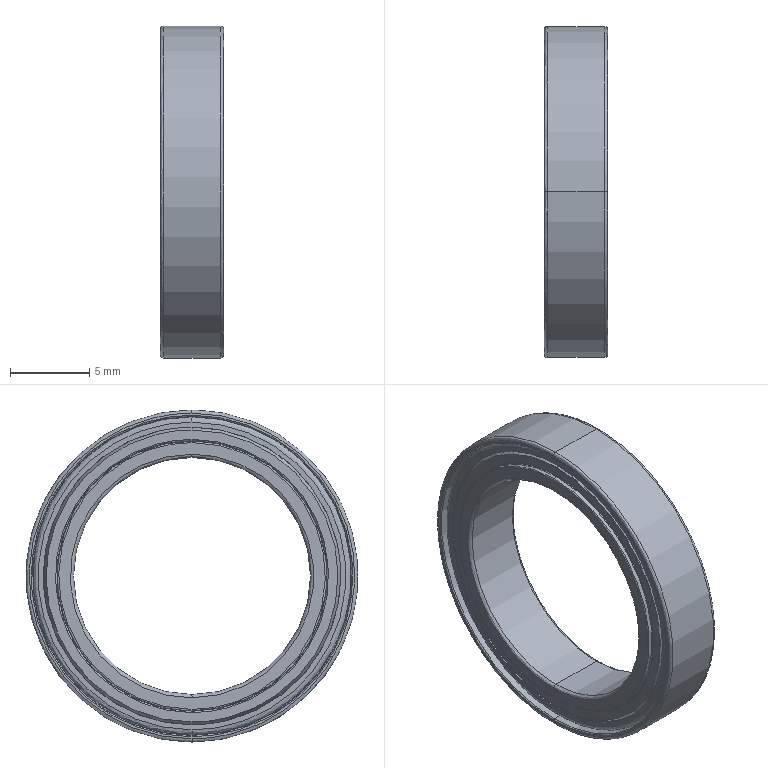Part | STEP file | Deep groove ball bearing NSK SB6702ZZ-1 | 1 solid | 136 faces | box 4 x 21 x 21 mm | volume 419.102 mm3 | spline 72 | cylinder 32 | plane 24 | cone 8 | commonest cylinder face diameters 16.73 x4 17 x4 17.14 x4 17.274 x4 20.2 x4 15 x2